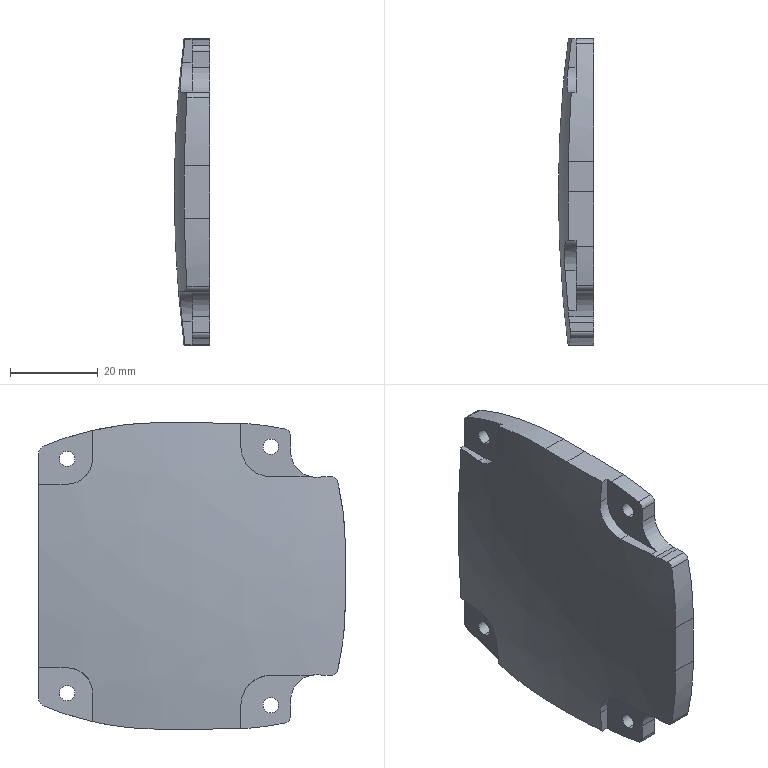Part | STEP file | _BMH070 Abschlussdeckel | 1 solid | 51 faces | box 8 x 70 x 70 mm | volume 28903 mm3 | cylinder 27 | plane 23 | spline 1 | commonest cylinder face diameters 3.5 x8 140 x6 3 x4 12 x3 4 x2 11.6 x2